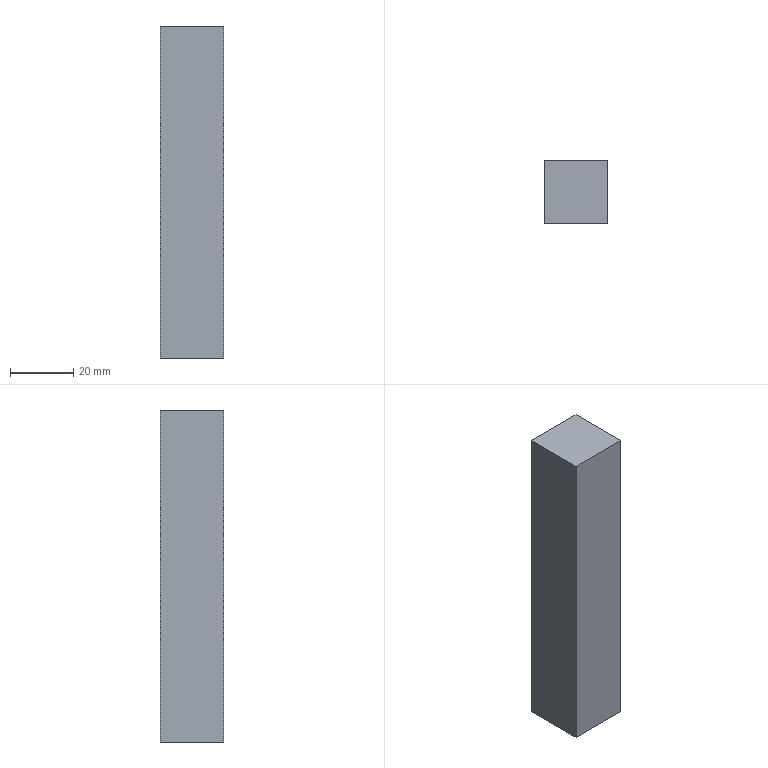Part | STEP file | 1 solid | 6 faces | box 20 x 20 x 105 mm | volume 42000 mm3 | plane 6
STEP:
#1=CARTESIAN_POINT('',(0.,0.,0.));
#2=DIRECTION('',(0.,0.,1.));
#3=DIRECTION('',(1.,0.,0.));
#4=AXIS2_PLACEMENT_3D('',#1,#2,#3);
#5=CARTESIAN_POINT('',(-135.363,70.5,253.53));
#6=VERTEX_POINT('',#5);
#7=CARTESIAN_POINT('',(-135.363,70.5,358.53));
#8=VERTEX_POINT('',#7);
#9=CARTESIAN_POINT('',(-135.363,70.5,-363.47));
#10=DIRECTION('',(0.,0.,1.));
#11=VECTOR('',#10,1.);
#12=LINE('',#9,#11);
#13=CARTESIAN_POINT('',(-155.363,70.5,-363.47));
#14=DIRECTION('',(0.,1.,0.));
#15=DIRECTION('',(0.,0.,1.));
#16=AXIS2_PLACEMENT_3D('',#13,#14,#15);
#17=PLANE('',#16);
#18=CARTESIAN_POINT('',(0.,20.));
#19=DIRECTION('',(1.,0.));
#20=VECTOR('',#19,1.);
#21=LINE('',#18,#20);
#22=(GEOMETRIC_REPRESENTATION_CONTEXT(2)PARAMETRIC_REPRESENTATION_CONTEXT()REPRESENTATION_CONTEXT('',''));
#23=DEFINITIONAL_REPRESENTATION('',(#21),#22);
#24=PCURVE('',#17,#23);
#25=CARTESIAN_POINT('',(-135.363,43.,253.53));
#26=DIRECTION('',(-1.,0.,0.));
#27=DIRECTION('',(0.,0.,1.));
#28=AXIS2_PLACEMENT_3D('',#25,#26,#27);
#29=PLANE('',#28);
#30=CARTESIAN_POINT('',(-617.,27.5));
#31=DIRECTION('',(1.,0.));
#32=VECTOR('',#31,1.);
#33=LINE('',#30,#32);
#34=(GEOMETRIC_REPRESENTATION_CONTEXT(2)PARAMETRIC_REPRESENTATION_CONTEXT()REPRESENTATION_CONTEXT('',''));
#35=DEFINITIONAL_REPRESENTATION('',(#33),#34);
#36=PCURVE('',#29,#35);
#37=SURFACE_CURVE('',#12,(#24,#36),.PCURVE_S1.);
#38=EDGE_CURVE('',#6,#8,#37,.T.);
#39=ORIENTED_EDGE('',*,*,#38,.T.);
#40=CARTESIAN_POINT('',(-155.363,70.5,358.53));
#41=VERTEX_POINT('',#40);
#42=CARTESIAN_POINT('',(-155.363,70.5,358.53));
#43=DIRECTION('',(1.,0.,0.));
#44=VECTOR('',#43,1.);
#45=LINE('',#42,#44);
#46=CARTESIAN_POINT('',(722.,0.));
#47=DIRECTION('',(0.,1.));
#48=VECTOR('',#47,1.);
#49=LINE('',#46,#48);
#50=(GEOMETRIC_REPRESENTATION_CONTEXT(2)PARAMETRIC_REPRESENTATION_CONTEXT()REPRESENTATION_CONTEXT('',''));
#51=DEFINITIONAL_REPRESENTATION('',(#49),#50);
#52=PCURVE('',#17,#51);
#53=CARTESIAN_POINT('',(-155.363,70.5,358.53));
#54=DIRECTION('',(0.,0.,-1.));
#55=DIRECTION('',(-1.,0.,0.));
#56=AXIS2_PLACEMENT_3D('',#53,#54,#55);
#57=PLANE('',#56);
#58=CARTESIAN_POINT('',(0.,0.));
#59=DIRECTION('',(-1.,0.));
#60=VECTOR('',#59,1.);
#61=LINE('',#58,#60);
#62=(GEOMETRIC_REPRESENTATION_CONTEXT(2)PARAMETRIC_REPRESENTATION_CONTEXT()REPRESENTATION_CONTEXT('',''));
#63=DEFINITIONAL_REPRESENTATION('',(#61),#62);
#64=PCURVE('',#57,#63);
#65=SURFACE_CURVE('',#45,(#52,#64),.PCURVE_S1.);
#66=EDGE_CURVE('',#41,#8,#65,.T.);
#67=ORIENTED_EDGE('',*,*,#66,.F.);
#68=CARTESIAN_POINT('',(-155.363,70.5,253.53));
#69=VERTEX_POINT('',#68);
#70=CARTESIAN_POINT('',(-155.363,70.5,-363.47));
#71=DIRECTION('',(0.,0.,1.));
#72=VECTOR('',#71,1.);
#73=LINE('',#70,#72);
#74=CARTESIAN_POINT('',(0.,0.));
#75=DIRECTION('',(1.,0.));
#76=VECTOR('',#75,1.);
#77=LINE('',#74,#76);
#78=(GEOMETRIC_REPRESENTATION_CONTEXT(2)PARAMETRIC_REPRESENTATION_CONTEXT()REPRESENTATION_CONTEXT('',''));
#79=DEFINITIONAL_REPRESENTATION('',(#77),#78);
#80=PCURVE('',#17,#79);
#81=CARTESIAN_POINT('',(-155.363,43.,253.53));
#82=DIRECTION('',(-1.,0.,0.));
#83=DIRECTION('',(0.,0.,1.));
#84=AXIS2_PLACEMENT_3D('',#81,#82,#83);
#85=PLANE('',#84);
#86=CARTESIAN_POINT('',(-617.,27.5));
#87=DIRECTION('',(1.,0.));
#88=VECTOR('',#87,1.);
#89=LINE('',#86,#88);
#90=(GEOMETRIC_REPRESENTATION_CONTEXT(2)PARAMETRIC_REPRESENTATION_CONTEXT()REPRESENTATION_CONTEXT('',''));
#91=DEFINITIONAL_REPRESENTATION('',(#89),#90);
#92=PCURVE('',#85,#91);
#93=SURFACE_CURVE('',#73,(#80,#92),.PCURVE_S1.);
#94=EDGE_CURVE('',#69,#41,#93,.T.);
#95=ORIENTED_EDGE('',*,*,#94,.F.);
#96=CARTESIAN_POINT('',(-155.363,70.5,253.53));
#97=DIRECTION('',(1.,0.,0.));
#98=VECTOR('',#97,1.);
#99=LINE('',#96,#98);
#100=CARTESIAN_POINT('',(617.,0.));
#101=DIRECTION('',(0.,1.));
#102=VECTOR('',#101,1.);
#103=LINE('',#100,#102);
#104=(GEOMETRIC_REPRESENTATION_CONTEXT(2)PARAMETRIC_REPRESENTATION_CONTEXT()REPRESENTATION_CONTEXT('',''));
#105=DEFINITIONAL_REPRESENTATION('',(#103),#104);
#106=PCURVE('',#17,#105);
#107=CARTESIAN_POINT('',(-155.363,43.,253.53));
#108=DIRECTION('',(0.,0.,1.));
#109=DIRECTION('',(1.,0.,0.));
#110=AXIS2_PLACEMENT_3D('',#107,#108,#109);
#111=PLANE('',#110);
#112=CARTESIAN_POINT('',(0.,27.5));
#113=DIRECTION('',(1.,0.));
#114=VECTOR('',#113,1.);
#115=LINE('',#112,#114);
#116=(GEOMETRIC_REPRESENTATION_CONTEXT(2)PARAMETRIC_REPRESENTATION_CONTEXT()REPRESENTATION_CONTEXT('',''));
#117=DEFINITIONAL_REPRESENTATION('',(#115),#116);
#118=PCURVE('',#111,#117);
#119=SURFACE_CURVE('',#99,(#106,#118),.PCURVE_S1.);
#120=EDGE_CURVE('',#69,#6,#119,.T.);
#121=ORIENTED_EDGE('',*,*,#120,.T.);
#122=EDGE_LOOP('',(#39,#67,#95,#121));
#123=FACE_BOUND('',#122,.T.);
#124=ADVANCED_FACE('',(#123),#17,.F.);
#125=CARTESIAN_POINT('',(-135.363,90.5,253.53));
#126=VERTEX_POINT('',#125);
#127=CARTESIAN_POINT('',(-135.363,43.,253.53));
#128=DIRECTION('',(0.,-1.,0.));
#129=VECTOR('',#128,1.);
#130=LINE('',#127,#129);
#131=CARTESIAN_POINT('',(20.,0.));
#132=DIRECTION('',(0.,-1.));
#133=VECTOR('',#132,1.);
#134=LINE('',#131,#133);
#135=(GEOMETRIC_REPRESENTATION_CONTEXT(2)PARAMETRIC_REPRESENTATION_CONTEXT()REPRESENTATION_CONTEXT('',''));
#136=DEFINITIONAL_REPRESENTATION('',(#134),#135);
#137=PCURVE('',#111,#136);
#138=CARTESIAN_POINT('',(0.,0.));
#139=DIRECTION('',(0.,-1.));
#140=VECTOR('',#139,1.);
#141=LINE('',#138,#140);
#142=(GEOMETRIC_REPRESENTATION_CONTEXT(2)PARAMETRIC_REPRESENTATION_CONTEXT()REPRESENTATION_CONTEXT('',''));
#143=DEFINITIONAL_REPRESENTATION('',(#141),#142);
#144=PCURVE('',#29,#143);
#145=SURFACE_CURVE('',#130,(#137,#144),.PCURVE_S1.);
#146=EDGE_CURVE('',#126,#6,#145,.T.);
#147=ORIENTED_EDGE('',*,*,#146,.T.);
#148=ORIENTED_EDGE('',*,*,#120,.F.);
#149=CARTESIAN_POINT('',(-155.363,90.5,253.53));
#150=VERTEX_POINT('',#149);
#151=CARTESIAN_POINT('',(-155.363,43.,253.53));
#152=DIRECTION('',(0.,-1.,0.));
#153=VECTOR('',#152,1.);
#154=LINE('',#151,#153);
#155=CARTESIAN_POINT('',(0.,0.));
#156=DIRECTION('',(0.,-1.));
#157=VECTOR('',#156,1.);
#158=LINE('',#155,#157);
#159=(GEOMETRIC_REPRESENTATION_CONTEXT(2)PARAMETRIC_REPRESENTATION_CONTEXT()REPRESENTATION_CONTEXT('',''));
#160=DEFINITIONAL_REPRESENTATION('',(#158),#159);
#161=PCURVE('',#111,#160);
#162=CARTESIAN_POINT('',(0.,0.));
#163=DIRECTION('',(0.,-1.));
#164=VECTOR('',#163,1.);
#165=LINE('',#162,#164);
#166=(GEOMETRIC_REPRESENTATION_CONTEXT(2)PARAMETRIC_REPRESENTATION_CONTEXT()REPRESENTATION_CONTEXT('',''));
#167=DEFINITIONAL_REPRESENTATION('',(#165),#166);
#168=PCURVE('',#85,#167);
#169=SURFACE_CURVE('',#154,(#161,#168),.PCURVE_S1.);
#170=EDGE_CURVE('',#150,#69,#169,.T.);
#171=ORIENTED_EDGE('',*,*,#170,.F.);
#172=CARTESIAN_POINT('',(-155.363,90.5,253.53));
#173=CARTESIAN_POINT('',(-148.696,90.5,253.53));
#174=CARTESIAN_POINT('',(-142.029,90.5,253.53));
#175=CARTESIAN_POINT('',(-135.363,90.5,253.53));
#176=B_SPLINE_CURVE_WITH_KNOTS('',3,(#172,#173,#174,#175),.UNSPECIFIED.,.F.,.F.,(4,4),(0.,1.),.PIECEWISE_BEZIER_KNOTS.);
#177=CARTESIAN_POINT('',(0.,47.5));
#178=CARTESIAN_POINT('',(6.667,47.5));
#179=CARTESIAN_POINT('',(13.333,47.5));
#180=CARTESIAN_POINT('',(20.,47.5));
#181=B_SPLINE_CURVE_WITH_KNOTS('',3,(#177,#178,#179,#180),.UNSPECIFIED.,.F.,.F.,(4,4),(0.,1.),.PIECEWISE_BEZIER_KNOTS.);
#182=(GEOMETRIC_REPRESENTATION_CONTEXT(2)PARAMETRIC_REPRESENTATION_CONTEXT()REPRESENTATION_CONTEXT('',''));
#183=DEFINITIONAL_REPRESENTATION('',(#181),#182);
#184=PCURVE('',#111,#183);
#185=CARTESIAN_POINT('',(-155.363,90.5,253.53));
#186=DIRECTION('',(0.,-1.,0.));
#187=DIRECTION('',(0.,0.,-1.));
#188=AXIS2_PLACEMENT_3D('',#185,#186,#187);
#189=PLANE('',#188);
#190=CARTESIAN_POINT('',(0.,0.));
#191=CARTESIAN_POINT('',(0.,6.667));
#192=CARTESIAN_POINT('',(0.,13.333));
#193=CARTESIAN_POINT('',(0.,20.));
#194=B_SPLINE_CURVE_WITH_KNOTS('',3,(#190,#191,#192,#193),.UNSPECIFIED.,.F.,.F.,(4,4),(0.,1.),.PIECEWISE_BEZIER_KNOTS.);
#195=(GEOMETRIC_REPRESENTATION_CONTEXT(2)PARAMETRIC_REPRESENTATION_CONTEXT()REPRESENTATION_CONTEXT('',''));
#196=DEFINITIONAL_REPRESENTATION('',(#194),#195);
#197=PCURVE('',#189,#196);
#198=SURFACE_CURVE('',#176,(#184,#197),.PCURVE_S1.);
#199=EDGE_CURVE('',#150,#126,#198,.T.);
#200=ORIENTED_EDGE('',*,*,#199,.T.);
#201=EDGE_LOOP('',(#147,#148,#171,#200));
#202=FACE_BOUND('',#201,.T.);
#203=ADVANCED_FACE('',(#202),#111,.F.);
#204=CARTESIAN_POINT('',(-135.363,90.5,358.53));
#205=VERTEX_POINT('',#204);
#206=CARTESIAN_POINT('',(-135.363,90.5,253.53));
#207=DIRECTION('',(0.,0.,-1.));
#208=VECTOR('',#207,1.);
#209=LINE('',#206,#208);
#210=CARTESIAN_POINT('',(0.,20.));
#211=DIRECTION('',(1.,0.));
#212=VECTOR('',#211,1.);
#213=LINE('',#210,#212);
#214=(GEOMETRIC_REPRESENTATION_CONTEXT(2)PARAMETRIC_REPRESENTATION_CONTEXT()REPRESENTATION_CONTEXT('',''));
#215=DEFINITIONAL_REPRESENTATION('',(#213),#214);
#216=PCURVE('',#189,#215);
#217=CARTESIAN_POINT('',(0.,47.5));
#218=DIRECTION('',(-1.,0.));
#219=VECTOR('',#218,1.);
#220=LINE('',#217,#219);
#221=(GEOMETRIC_REPRESENTATION_CONTEXT(2)PARAMETRIC_REPRESENTATION_CONTEXT()REPRESENTATION_CONTEXT('',''));
#222=DEFINITIONAL_REPRESENTATION('',(#220),#221);
#223=PCURVE('',#29,#222);
#224=SURFACE_CURVE('',#209,(#216,#223),.PCURVE_S1.);
#225=EDGE_CURVE('',#205,#126,#224,.T.);
#226=ORIENTED_EDGE('',*,*,#225,.T.);
#227=ORIENTED_EDGE('',*,*,#199,.F.);
#228=CARTESIAN_POINT('',(-155.363,90.5,358.53));
#229=VERTEX_POINT('',#228);
#230=CARTESIAN_POINT('',(-155.363,90.5,253.53));
#231=DIRECTION('',(0.,0.,-1.));
#232=VECTOR('',#231,1.);
#233=LINE('',#230,#232);
#234=CARTESIAN_POINT('',(0.,0.));
#235=DIRECTION('',(1.,0.));
#236=VECTOR('',#235,1.);
#237=LINE('',#234,#236);
#238=(GEOMETRIC_REPRESENTATION_CONTEXT(2)PARAMETRIC_REPRESENTATION_CONTEXT()REPRESENTATION_CONTEXT('',''));
#239=DEFINITIONAL_REPRESENTATION('',(#237),#238);
#240=PCURVE('',#189,#239);
#241=CARTESIAN_POINT('',(0.,47.5));
#242=DIRECTION('',(-1.,0.));
#243=VECTOR('',#242,1.);
#244=LINE('',#241,#243);
#245=(GEOMETRIC_REPRESENTATION_CONTEXT(2)PARAMETRIC_REPRESENTATION_CONTEXT()REPRESENTATION_CONTEXT('',''));
#246=DEFINITIONAL_REPRESENTATION('',(#244),#245);
#247=PCURVE('',#85,#246);
#248=SURFACE_CURVE('',#233,(#240,#247),.PCURVE_S1.);
#249=EDGE_CURVE('',#229,#150,#248,.T.);
#250=ORIENTED_EDGE('',*,*,#249,.F.);
#251=CARTESIAN_POINT('',(-155.363,90.5,358.53));
#252=DIRECTION('',(1.,0.,0.));
#253=VECTOR('',#252,1.);
#254=LINE('',#251,#253);
#255=CARTESIAN_POINT('',(-105.,0.));
#256=DIRECTION('',(0.,1.));
#257=VECTOR('',#256,1.);
#258=LINE('',#255,#257);
#259=(GEOMETRIC_REPRESENTATION_CONTEXT(2)PARAMETRIC_REPRESENTATION_CONTEXT()REPRESENTATION_CONTEXT('',''));
#260=DEFINITIONAL_REPRESENTATION('',(#258),#259);
#261=PCURVE('',#189,#260);
#262=CARTESIAN_POINT('',(0.,20.));
#263=DIRECTION('',(-1.,0.));
#264=VECTOR('',#263,1.);
#265=LINE('',#262,#264);
#266=(GEOMETRIC_REPRESENTATION_CONTEXT(2)PARAMETRIC_REPRESENTATION_CONTEXT()REPRESENTATION_CONTEXT('',''));
#267=DEFINITIONAL_REPRESENTATION('',(#265),#266);
#268=PCURVE('',#57,#267);
#269=SURFACE_CURVE('',#254,(#261,#268),.PCURVE_S1.);
#270=EDGE_CURVE('',#229,#205,#269,.T.);
#271=ORIENTED_EDGE('',*,*,#270,.T.);
#272=EDGE_LOOP('',(#226,#227,#250,#271));
#273=FACE_BOUND('',#272,.T.);
#274=ADVANCED_FACE('',(#273),#189,.F.);
#275=CARTESIAN_POINT('',(-135.363,70.5,358.53));
#276=DIRECTION('',(0.,1.,0.));
#277=VECTOR('',#276,1.);
#278=LINE('',#275,#277);
#279=CARTESIAN_POINT('',(-20.,0.));
#280=DIRECTION('',(0.,1.));
#281=VECTOR('',#280,1.);
#282=LINE('',#279,#281);
#283=(GEOMETRIC_REPRESENTATION_CONTEXT(2)PARAMETRIC_REPRESENTATION_CONTEXT()REPRESENTATION_CONTEXT('',''));
#284=DEFINITIONAL_REPRESENTATION('',(#282),#283);
#285=PCURVE('',#57,#284);
#286=CARTESIAN_POINT('',(105.,27.5));
#287=DIRECTION('',(0.,1.));
#288=VECTOR('',#287,1.);
#289=LINE('',#286,#288);
#290=(GEOMETRIC_REPRESENTATION_CONTEXT(2)PARAMETRIC_REPRESENTATION_CONTEXT()REPRESENTATION_CONTEXT('',''));
#291=DEFINITIONAL_REPRESENTATION('',(#289),#290);
#292=PCURVE('',#29,#291);
#293=SURFACE_CURVE('',#278,(#285,#292),.PCURVE_S1.);
#294=EDGE_CURVE('',#8,#205,#293,.T.);
#295=ORIENTED_EDGE('',*,*,#294,.T.);
#296=ORIENTED_EDGE('',*,*,#270,.F.);
#297=CARTESIAN_POINT('',(-155.363,70.5,358.53));
#298=DIRECTION('',(0.,1.,0.));
#299=VECTOR('',#298,1.);
#300=LINE('',#297,#299);
#301=CARTESIAN_POINT('',(0.,0.));
#302=DIRECTION('',(0.,1.));
#303=VECTOR('',#302,1.);
#304=LINE('',#301,#303);
#305=(GEOMETRIC_REPRESENTATION_CONTEXT(2)PARAMETRIC_REPRESENTATION_CONTEXT()REPRESENTATION_CONTEXT('',''));
#306=DEFINITIONAL_REPRESENTATION('',(#304),#305);
#307=PCURVE('',#57,#306);
#308=CARTESIAN_POINT('',(105.,27.5));
#309=DIRECTION('',(0.,1.));
#310=VECTOR('',#309,1.);
#311=LINE('',#308,#310);
#312=(GEOMETRIC_REPRESENTATION_CONTEXT(2)PARAMETRIC_REPRESENTATION_CONTEXT()REPRESENTATION_CONTEXT('',''));
#313=DEFINITIONAL_REPRESENTATION('',(#311),#312);
#314=PCURVE('',#85,#313);
#315=SURFACE_CURVE('',#300,(#307,#314),.PCURVE_S1.);
#316=EDGE_CURVE('',#41,#229,#315,.T.);
#317=ORIENTED_EDGE('',*,*,#316,.F.);
#318=ORIENTED_EDGE('',*,*,#66,.T.);
#319=EDGE_LOOP('',(#295,#296,#317,#318));
#320=FACE_BOUND('',#319,.T.);
#321=ADVANCED_FACE('',(#320),#57,.F.);
#322=ORIENTED_EDGE('',*,*,#94,.T.);
#323=ORIENTED_EDGE('',*,*,#316,.T.);
#324=ORIENTED_EDGE('',*,*,#249,.T.);
#325=ORIENTED_EDGE('',*,*,#170,.T.);
#326=EDGE_LOOP('',(#322,#323,#324,#325));
#327=FACE_BOUND('',#326,.T.);
#328=ADVANCED_FACE('',(#327),#85,.T.);
#329=ORIENTED_EDGE('',*,*,#38,.F.);
#330=ORIENTED_EDGE('',*,*,#146,.F.);
#331=ORIENTED_EDGE('',*,*,#225,.F.);
#332=ORIENTED_EDGE('',*,*,#294,.F.);
#333=EDGE_LOOP('',(#329,#330,#331,#332));
#334=FACE_BOUND('',#333,.T.);
#335=ADVANCED_FACE('',(#334),#29,.F.);
#336=CLOSED_SHELL('',(#124,#203,#274,#321,#328,#335));
#337=MANIFOLD_SOLID_BREP('',#336);
#338=(LENGTH_UNIT()NAMED_UNIT(*)SI_UNIT(.MILLI.,.METRE.));
#339=UNCERTAINTY_MEASURE_WITH_UNIT(LENGTH_MEASURE(0.0000001),#338,'','');
#340=(NAMED_UNIT(*)PLANE_ANGLE_UNIT()SI_UNIT($,.RADIAN.));
#341=(NAMED_UNIT(*)SI_UNIT($,.STERADIAN.)SOLID_ANGLE_UNIT());
#342=(GEOMETRIC_REPRESENTATION_CONTEXT(3)GLOBAL_UNCERTAINTY_ASSIGNED_CONTEXT((#339))GLOBAL_UNIT_ASSIGNED_CONTEXT((#338,#340,#341))REPRESENTATION_CONTEXT('',''));
#343=ADVANCED_BREP_SHAPE_REPRESENTATION('',(#4,#337),#342);